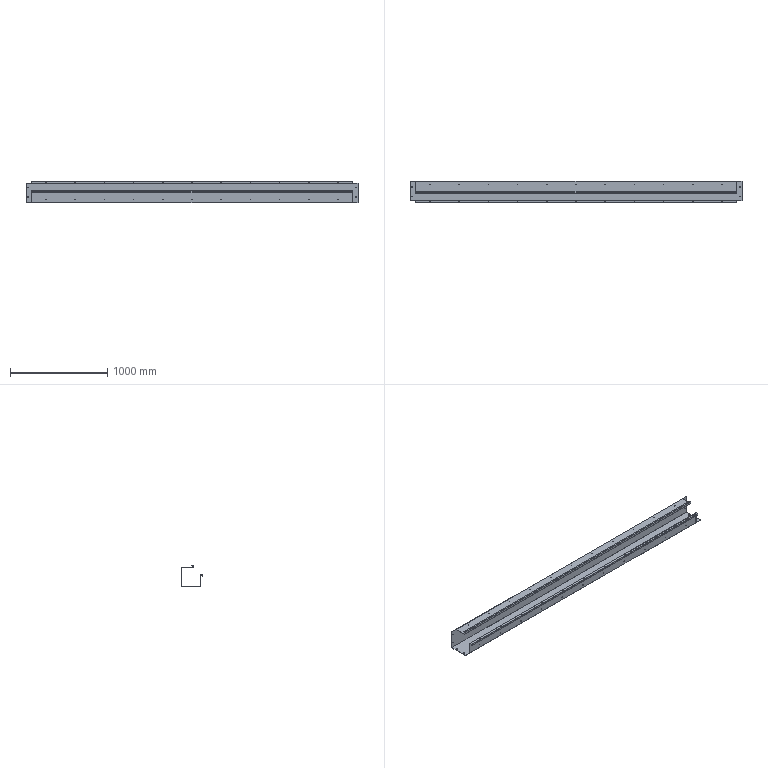Part | STEP file | SX-S01 | 1 solid | 237 faces | box 3411 x 223 x 223 mm | volume 4765265 mm3 | cylinder 129 | plane 108 | commonest cylinder face diameters 8 x55 5.4 x44 7 x16 0.4 x7 4.4 x7